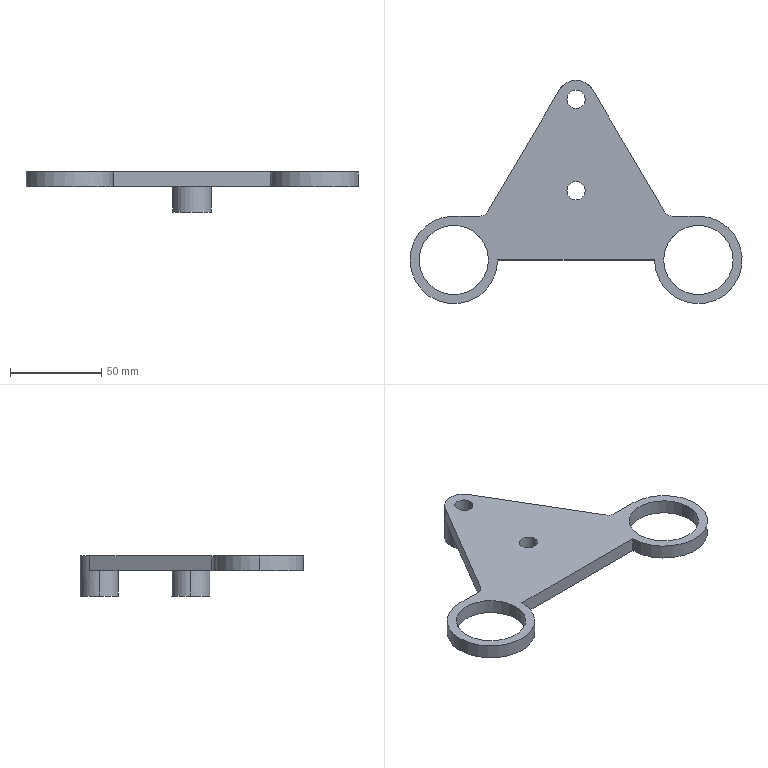Part | SolidWorks | features Extrusion 1, ICE 1 | 1 solid | 26 faces | box 182 x 122.5 x 22 mm | volume 68800 mm3 | cylinder 17 | plane 9 | commonest cylinder face diameters 10 x6 21 x4 38 x4 48 x3
STEP:
#1=CARTESIAN_POINT('',(-10.5,38.,-14.));
#2=VERTEX_POINT('',#1);
#3=CARTESIAN_POINT('',(10.5,38.,-14.));
#4=VERTEX_POINT('',#3);
#5=CARTESIAN_POINT('',(0.,38.,-14.));
#6=DIRECTION('',(0.,0.,-1.));
#7=DIRECTION('',(-1.,0.,0.));
#8=AXIS2_PLACEMENT_3D('',#5,#6,#7);
#9=CIRCLE('',#8,10.5);
#10=EDGE_CURVE('',#2,#4,#9,.T.);
#11=ORIENTED_EDGE('',*,*,#10,.F.);
#12=CARTESIAN_POINT('',(-10.5,38.,0.));
#13=VERTEX_POINT('',#12);
#14=CARTESIAN_POINT('',(-10.5,38.,-14.));
#15=DIRECTION('',(0.,0.,1.));
#16=VECTOR('',#15,1000.);
#17=LINE('',#14,#16);
#18=EDGE_CURVE('',#2,#13,#17,.T.);
#19=ORIENTED_EDGE('',*,*,#18,.T.);
#20=CARTESIAN_POINT('',(10.5,38.,0.));
#21=VERTEX_POINT('',#20);
#22=CARTESIAN_POINT('',(0.,38.,0.));
#23=DIRECTION('',(0.,0.,-1.));
#24=DIRECTION('',(1.,0.,0.));
#25=AXIS2_PLACEMENT_3D('',#22,#23,#24);
#26=CIRCLE('',#25,10.5);
#27=EDGE_CURVE('',#13,#21,#26,.T.);
#28=ORIENTED_EDGE('',*,*,#27,.T.);
#29=CARTESIAN_POINT('',(10.5,38.,-14.));
#30=DIRECTION('',(0.,0.,1.));
#31=VECTOR('',#30,1000.);
#32=LINE('',#29,#31);
#33=EDGE_CURVE('',#4,#21,#32,.T.);
#34=ORIENTED_EDGE('',*,*,#33,.F.);
#35=EDGE_LOOP('',(#11,#19,#28,#34));
#36=FACE_OUTER_BOUND('',#35,.T.);
#37=CARTESIAN_POINT('',(0.,38.,-14.));
#38=DIRECTION('',(0.,0.,1.));
#39=DIRECTION('',(1.,0.,0.));
#40=AXIS2_PLACEMENT_3D('',#37,#38,#39);
#41=CYLINDRICAL_SURFACE('',#40,10.5);
#42=ADVANCED_FACE('',(#36),#41,.T.);
#43=CARTESIAN_POINT('',(-5.,38.,8.));
#44=VERTEX_POINT('',#43);
#45=CARTESIAN_POINT('',(5.,38.,8.));
#46=VERTEX_POINT('',#45);
#47=CARTESIAN_POINT('',(0.,38.,8.));
#48=DIRECTION('',(0.,0.,1.));
#49=DIRECTION('',(1.,0.,0.));
#50=AXIS2_PLACEMENT_3D('',#47,#48,#49);
#51=CIRCLE('',#50,5.);
#52=EDGE_CURVE('',#44,#46,#51,.T.);
#53=ORIENTED_EDGE('',*,*,#52,.T.);
#54=CARTESIAN_POINT('',(5.,38.,-14.));
#55=VERTEX_POINT('',#54);
#56=CARTESIAN_POINT('',(5.,38.,8.));
#57=DIRECTION('',(0.,0.,-1.));
#58=VECTOR('',#57,1000.);
#59=LINE('',#56,#58);
#60=EDGE_CURVE('',#46,#55,#59,.T.);
#61=ORIENTED_EDGE('',*,*,#60,.T.);
#62=CARTESIAN_POINT('',(-5.,38.,-14.));
#63=VERTEX_POINT('',#62);
#64=CARTESIAN_POINT('',(0.,38.,-14.));
#65=DIRECTION('',(0.,0.,-1.));
#66=DIRECTION('',(-1.,0.,0.));
#67=AXIS2_PLACEMENT_3D('',#64,#65,#66);
#68=CIRCLE('',#67,5.);
#69=EDGE_CURVE('',#55,#63,#68,.T.);
#70=ORIENTED_EDGE('',*,*,#69,.T.);
#71=CARTESIAN_POINT('',(-5.,38.,8.));
#72=DIRECTION('',(0.,0.,-1.));
#73=VECTOR('',#72,1000.);
#74=LINE('',#71,#73);
#75=EDGE_CURVE('',#44,#63,#74,.T.);
#76=ORIENTED_EDGE('',*,*,#75,.F.);
#77=EDGE_LOOP('',(#53,#61,#70,#76));
#78=FACE_OUTER_BOUND('',#77,.T.);
#79=CARTESIAN_POINT('',(0.,38.,8.));
#80=DIRECTION('',(0.,0.,-1.));
#81=DIRECTION('',(-1.,0.,0.));
#82=AXIS2_PLACEMENT_3D('',#79,#80,#81);
#83=CYLINDRICAL_SURFACE('',#82,5.);
#84=ADVANCED_FACE('',(#78),#83,.F.);
#85=CARTESIAN_POINT('',(-5.,88.,8.));
#86=VERTEX_POINT('',#85);
#87=CARTESIAN_POINT('',(5.,88.,8.));
#88=VERTEX_POINT('',#87);
#89=CARTESIAN_POINT('',(0.,88.,8.));
#90=DIRECTION('',(0.,0.,1.));
#91=DIRECTION('',(1.,0.,0.));
#92=AXIS2_PLACEMENT_3D('',#89,#90,#91);
#93=CIRCLE('',#92,5.);
#94=EDGE_CURVE('',#86,#88,#93,.T.);
#95=ORIENTED_EDGE('',*,*,#94,.T.);
#96=CARTESIAN_POINT('',(5.,88.,-14.));
#97=VERTEX_POINT('',#96);
#98=CARTESIAN_POINT('',(5.,88.,8.));
#99=DIRECTION('',(0.,0.,-1.));
#100=VECTOR('',#99,1000.);
#101=LINE('',#98,#100);
#102=EDGE_CURVE('',#88,#97,#101,.T.);
#103=ORIENTED_EDGE('',*,*,#102,.T.);
#104=CARTESIAN_POINT('',(-5.,88.,-14.));
#105=VERTEX_POINT('',#104);
#106=CARTESIAN_POINT('',(0.,88.,-14.));
#107=DIRECTION('',(0.,0.,-1.));
#108=DIRECTION('',(-1.,0.,0.));
#109=AXIS2_PLACEMENT_3D('',#106,#107,#108);
#110=CIRCLE('',#109,5.);
#111=EDGE_CURVE('',#97,#105,#110,.T.);
#112=ORIENTED_EDGE('',*,*,#111,.T.);
#113=CARTESIAN_POINT('',(-5.,88.,8.));
#114=DIRECTION('',(0.,0.,-1.));
#115=VECTOR('',#114,1000.);
#116=LINE('',#113,#115);
#117=EDGE_CURVE('',#86,#105,#116,.T.);
#118=ORIENTED_EDGE('',*,*,#117,.F.);
#119=EDGE_LOOP('',(#95,#103,#112,#118));
#120=FACE_OUTER_BOUND('',#119,.T.);
#121=CARTESIAN_POINT('',(0.,88.,8.));
#122=DIRECTION('',(0.,0.,-1.));
#123=DIRECTION('',(-1.,0.,0.));
#124=AXIS2_PLACEMENT_3D('',#121,#122,#123);
#125=CYLINDRICAL_SURFACE('',#124,5.);
#126=ADVANCED_FACE('',(#120),#125,.F.);
#127=CARTESIAN_POINT('',(86.,0.,8.));
#128=VERTEX_POINT('',#127);
#129=CARTESIAN_POINT('',(48.,0.,8.));
#130=VERTEX_POINT('',#129);
#131=CARTESIAN_POINT('',(67.,0.,8.));
#132=DIRECTION('',(0.,0.,-1.));
#133=DIRECTION('',(1.,0.,0.));
#134=AXIS2_PLACEMENT_3D('',#131,#132,#133);
#135=CIRCLE('',#134,19.);
#136=EDGE_CURVE('',#128,#130,#135,.T.);
#137=ORIENTED_EDGE('',*,*,#136,.F.);
#138=CARTESIAN_POINT('',(86.,0.,0.));
#139=VERTEX_POINT('',#138);
#140=CARTESIAN_POINT('',(86.,0.,8.));
#141=DIRECTION('',(0.,0.,-1.));
#142=VECTOR('',#141,1000.);
#143=LINE('',#140,#142);
#144=EDGE_CURVE('',#128,#139,#143,.T.);
#145=ORIENTED_EDGE('',*,*,#144,.T.);
#146=CARTESIAN_POINT('',(48.,0.,0.));
#147=VERTEX_POINT('',#146);
#148=CARTESIAN_POINT('',(67.,0.,0.));
#149=DIRECTION('',(0.,0.,-1.));
#150=DIRECTION('',(1.,0.,0.));
#151=AXIS2_PLACEMENT_3D('',#148,#149,#150);
#152=CIRCLE('',#151,19.);
#153=EDGE_CURVE('',#139,#147,#152,.T.);
#154=ORIENTED_EDGE('',*,*,#153,.T.);
#155=CARTESIAN_POINT('',(48.,0.,8.));
#156=DIRECTION('',(0.,0.,-1.));
#157=VECTOR('',#156,1000.);
#158=LINE('',#155,#157);
#159=EDGE_CURVE('',#130,#147,#158,.T.);
#160=ORIENTED_EDGE('',*,*,#159,.F.);
#161=EDGE_LOOP('',(#137,#145,#154,#160));
#162=FACE_OUTER_BOUND('',#161,.T.);
#163=CARTESIAN_POINT('',(67.,0.,8.));
#164=DIRECTION('',(0.,0.,-1.));
#165=DIRECTION('',(-1.,0.,0.));
#166=AXIS2_PLACEMENT_3D('',#163,#164,#165);
#167=CYLINDRICAL_SURFACE('',#166,19.);
#168=ADVANCED_FACE('',(#162),#167,.F.);
#169=CARTESIAN_POINT('',(-86.,0.,8.));
#170=VERTEX_POINT('',#169);
#171=CARTESIAN_POINT('',(-48.,0.,8.));
#172=VERTEX_POINT('',#171);
#173=CARTESIAN_POINT('',(-67.,0.,8.));
#174=DIRECTION('',(0.,0.,1.));
#175=DIRECTION('',(1.,0.,0.));
#176=AXIS2_PLACEMENT_3D('',#173,#174,#175);
#177=CIRCLE('',#176,19.);
#178=EDGE_CURVE('',#170,#172,#177,.T.);
#179=ORIENTED_EDGE('',*,*,#178,.T.);
#180=CARTESIAN_POINT('',(-48.,0.,0.));
#181=VERTEX_POINT('',#180);
#182=CARTESIAN_POINT('',(-48.,0.,8.));
#183=DIRECTION('',(0.,0.,-1.));
#184=VECTOR('',#183,1000.);
#185=LINE('',#182,#184);
#186=EDGE_CURVE('',#172,#181,#185,.T.);
#187=ORIENTED_EDGE('',*,*,#186,.T.);
#188=CARTESIAN_POINT('',(-86.,0.,0.));
#189=VERTEX_POINT('',#188);
#190=CARTESIAN_POINT('',(-67.,0.,0.));
#191=DIRECTION('',(0.,0.,1.));
#192=DIRECTION('',(1.,0.,0.));
#193=AXIS2_PLACEMENT_3D('',#190,#191,#192);
#194=CIRCLE('',#193,19.);
#195=EDGE_CURVE('',#189,#181,#194,.T.);
#196=ORIENTED_EDGE('',*,*,#195,.F.);
#197=CARTESIAN_POINT('',(-86.,0.,8.));
#198=DIRECTION('',(0.,0.,-1.));
#199=VECTOR('',#198,1000.);
#200=LINE('',#197,#199);
#201=EDGE_CURVE('',#170,#189,#200,.T.);
#202=ORIENTED_EDGE('',*,*,#201,.F.);
#203=EDGE_LOOP('',(#179,#187,#196,#202));
#204=FACE_OUTER_BOUND('',#203,.T.);
#205=CARTESIAN_POINT('',(-67.,0.,8.));
#206=DIRECTION('',(0.,0.,-1.));
#207=DIRECTION('',(-1.,0.,0.));
#208=AXIS2_PLACEMENT_3D('',#205,#206,#207);
#209=CYLINDRICAL_SURFACE('',#208,19.);
#210=ADVANCED_FACE('',(#204),#209,.F.);
#211=CARTESIAN_POINT('',(-91.,0.,8.));
#212=VERTEX_POINT('',#211);
#213=CARTESIAN_POINT('',(-43.,0.,8.));
#214=VERTEX_POINT('',#213);
#215=CARTESIAN_POINT('',(-67.,0.,8.));
#216=DIRECTION('',(0.,0.,1.));
#217=DIRECTION('',(1.,0.,0.));
#218=AXIS2_PLACEMENT_3D('',#215,#216,#217);
#219=CIRCLE('',#218,24.);
#220=EDGE_CURVE('',#212,#214,#219,.T.);
#221=ORIENTED_EDGE('',*,*,#220,.F.);
#222=CARTESIAN_POINT('',(-91.,0.,0.));
#223=VERTEX_POINT('',#222);
#224=CARTESIAN_POINT('',(-91.,0.,8.));
#225=DIRECTION('',(0.,0.,-1.));
#226=VECTOR('',#225,1000.);
#227=LINE('',#224,#226);
#228=EDGE_CURVE('',#212,#223,#227,.T.);
#229=ORIENTED_EDGE('',*,*,#228,.T.);
#230=CARTESIAN_POINT('',(-43.,0.,0.));
#231=VERTEX_POINT('',#230);
#232=CARTESIAN_POINT('',(-67.,0.,0.));
#233=DIRECTION('',(0.,0.,1.));
#234=DIRECTION('',(1.,0.,0.));
#235=AXIS2_PLACEMENT_3D('',#232,#233,#234);
#236=CIRCLE('',#235,24.);
#237=EDGE_CURVE('',#223,#231,#236,.T.);
#238=ORIENTED_EDGE('',*,*,#237,.T.);
#239=CARTESIAN_POINT('',(-43.,0.,8.));
#240=DIRECTION('',(0.,0.,-1.));
#241=VECTOR('',#240,1000.);
#242=LINE('',#239,#241);
#243=EDGE_CURVE('',#214,#231,#242,.T.);
#244=ORIENTED_EDGE('',*,*,#243,.F.);
#245=EDGE_LOOP('',(#221,#229,#238,#244));
#246=FACE_OUTER_BOUND('',#245,.T.);
#247=CARTESIAN_POINT('',(-67.,0.,8.));
#248=DIRECTION('',(0.,0.,-1.));
#249=DIRECTION('',(-1.,0.,0.));
#250=AXIS2_PLACEMENT_3D('',#247,#248,#249);
#251=CYLINDRICAL_SURFACE('',#250,24.);
#252=ADVANCED_FACE('',(#246),#251,.T.);
#253=CARTESIAN_POINT('',(9.093,93.25,0.));
#254=VERTEX_POINT('',#253);
#255=CARTESIAN_POINT('',(10.5,88.,0.));
#256=VERTEX_POINT('',#255);
#257=CARTESIAN_POINT('',(0.,88.,0.));
#258=DIRECTION('',(0.,0.,-1.));
#259=DIRECTION('',(-1.,0.,0.));
#260=AXIS2_PLACEMENT_3D('',#257,#258,#259);
#261=CIRCLE('',#260,10.5);
#262=EDGE_CURVE('',#254,#256,#261,.T.);
#263=ORIENTED_EDGE('',*,*,#262,.T.);
#264=CARTESIAN_POINT('',(10.5,88.,-14.));
#265=VERTEX_POINT('',#264);
#266=CARTESIAN_POINT('',(10.5,88.,8.));
#267=DIRECTION('',(0.,0.,-1.));
#268=VECTOR('',#267,1000.);
#269=LINE('',#266,#268);
#270=EDGE_CURVE('',#256,#265,#269,.T.);
#271=ORIENTED_EDGE('',*,*,#270,.T.);
#272=CARTESIAN_POINT('',(-10.5,88.,-14.));
#273=VERTEX_POINT('',#272);
#274=CARTESIAN_POINT('',(0.,88.,-14.));
#275=DIRECTION('',(0.,0.,-1.));
#276=DIRECTION('',(-1.,0.,0.));
#277=AXIS2_PLACEMENT_3D('',#274,#275,#276);
#278=CIRCLE('',#277,10.5);
#279=EDGE_CURVE('',#273,#265,#278,.T.);
#280=ORIENTED_EDGE('',*,*,#279,.F.);
#281=CARTESIAN_POINT('',(-10.5,88.,0.));
#282=VERTEX_POINT('',#281);
#283=CARTESIAN_POINT('',(-10.5,88.,8.));
#284=DIRECTION('',(0.,0.,-1.));
#285=VECTOR('',#284,1000.);
#286=LINE('',#283,#285);
#287=EDGE_CURVE('',#282,#273,#286,.T.);
#288=ORIENTED_EDGE('',*,*,#287,.F.);
#289=CARTESIAN_POINT('',(-9.093,93.25,0.));
#290=VERTEX_POINT('',#289);
#291=CARTESIAN_POINT('',(0.,88.,0.));
#292=DIRECTION('',(0.,0.,-1.));
#293=DIRECTION('',(-1.,0.,0.));
#294=AXIS2_PLACEMENT_3D('',#291,#292,#293);
#295=CIRCLE('',#294,10.5);
#296=EDGE_CURVE('',#282,#290,#295,.T.);
#297=ORIENTED_EDGE('',*,*,#296,.T.);
#298=CARTESIAN_POINT('',(-9.093,93.25,8.));
#299=VERTEX_POINT('',#298);
#300=CARTESIAN_POINT('',(-9.093,93.25,8.));
#301=DIRECTION('',(0.,0.,-1.));
#302=VECTOR('',#301,1000.);
#303=LINE('',#300,#302);
#304=EDGE_CURVE('',#299,#290,#303,.T.);
#305=ORIENTED_EDGE('',*,*,#304,.F.);
#306=CARTESIAN_POINT('',(9.093,93.25,8.));
#307=VERTEX_POINT('',#306);
#308=CARTESIAN_POINT('',(0.,88.,8.));
#309=DIRECTION('',(0.,0.,1.));
#310=DIRECTION('',(1.,0.,0.));
#311=AXIS2_PLACEMENT_3D('',#308,#309,#310);
#312=CIRCLE('',#311,10.5);
#313=EDGE_CURVE('',#307,#299,#312,.T.);
#314=ORIENTED_EDGE('',*,*,#313,.F.);
#315=CARTESIAN_POINT('',(9.093,93.25,8.));
#316=DIRECTION('',(0.,0.,-1.));
#317=VECTOR('',#316,1000.);
#318=LINE('',#315,#317);
#319=EDGE_CURVE('',#307,#254,#318,.T.);
#320=ORIENTED_EDGE('',*,*,#319,.T.);
#321=EDGE_LOOP('',(#263,#271,#280,#288,#297,#305,#314,#320));
#322=FACE_OUTER_BOUND('',#321,.T.);
#323=CARTESIAN_POINT('',(0.,88.,8.));
#324=DIRECTION('',(0.,0.,-1.));
#325=DIRECTION('',(-1.,0.,0.));
#326=AXIS2_PLACEMENT_3D('',#323,#324,#325);
#327=CYLINDRICAL_SURFACE('',#326,10.5);
#328=ADVANCED_FACE('',(#322),#327,.T.);
#329=ORIENTED_EDGE('',*,*,#195,.T.);
#330=CARTESIAN_POINT('',(-67.,0.,0.));
#331=DIRECTION('',(0.,0.,1.));
#332=DIRECTION('',(1.,0.,0.));
#333=AXIS2_PLACEMENT_3D('',#330,#331,#332);
#334=CIRCLE('',#333,19.);
#335=EDGE_CURVE('',#181,#189,#334,.T.);
#336=ORIENTED_EDGE('',*,*,#335,.T.);
#337=EDGE_LOOP('',(#329,#336));
#338=FACE_BOUND('',#337,.T.);
#339=CARTESIAN_POINT('',(67.,0.,0.));
#340=DIRECTION('',(0.,0.,-1.));
#341=DIRECTION('',(1.,0.,0.));
#342=AXIS2_PLACEMENT_3D('',#339,#340,#341);
#343=CIRCLE('',#342,19.);
#344=EDGE_CURVE('',#147,#139,#343,.T.);
#345=ORIENTED_EDGE('',*,*,#344,.F.);
#346=ORIENTED_EDGE('',*,*,#153,.F.);
#347=EDGE_LOOP('',(#345,#346));
#348=FACE_BOUND('',#347,.T.);
#349=ORIENTED_EDGE('',*,*,#262,.F.);
#350=CARTESIAN_POINT('',(48.477,26.46,0.));
#351=VERTEX_POINT('',#350);
#352=CARTESIAN_POINT('',(47.547,28.037,0.));
#353=DIRECTION('',(0.5079,-0.8614,0.));
#354=VECTOR('',#353,1000.);
#355=LINE('',#352,#354);
#356=EDGE_CURVE('',#254,#351,#355,.T.);
#357=ORIENTED_EDGE('',*,*,#356,.T.);
#358=CARTESIAN_POINT('',(52.82,24.,0.));
#359=VERTEX_POINT('',#358);
#360=CARTESIAN_POINT('',(52.785,29.,0.));
#361=DIRECTION('',(0.,0.,-1.));
#362=DIRECTION('',(1.,0.,0.));
#363=AXIS2_PLACEMENT_3D('',#360,#361,#362);
#364=CIRCLE('',#363,5.);
#365=EDGE_CURVE('',#359,#351,#364,.T.);
#366=ORIENTED_EDGE('',*,*,#365,.F.);
#367=CARTESIAN_POINT('',(67.,24.,0.));
#368=VERTEX_POINT('',#367);
#369=CARTESIAN_POINT('',(0.,24.,0.));
#370=DIRECTION('',(-1.,0.,0.));
#371=VECTOR('',#370,1000.);
#372=LINE('',#369,#371);
#373=EDGE_CURVE('',#368,#359,#372,.T.);
#374=ORIENTED_EDGE('',*,*,#373,.F.);
#375=CARTESIAN_POINT('',(43.,0.,0.));
#376=VERTEX_POINT('',#375);
#377=CARTESIAN_POINT('',(67.,0.,0.));
#378=DIRECTION('',(0.,0.,-1.));
#379=DIRECTION('',(1.,0.,0.));
#380=AXIS2_PLACEMENT_3D('',#377,#378,#379);
#381=CIRCLE('',#380,24.);
#382=EDGE_CURVE('',#368,#376,#381,.T.);
#383=ORIENTED_EDGE('',*,*,#382,.T.);
#384=CARTESIAN_POINT('',(0.,0.,0.));
#385=DIRECTION('',(1.,0.,0.));
#386=VECTOR('',#385,1000.);
#387=LINE('',#384,#386);
#388=EDGE_CURVE('',#231,#376,#387,.T.);
#389=ORIENTED_EDGE('',*,*,#388,.F.);
#390=ORIENTED_EDGE('',*,*,#237,.F.);
#391=CARTESIAN_POINT('',(-67.,24.,0.));
#392=VERTEX_POINT('',#391);
#393=CARTESIAN_POINT('',(-67.,0.,0.));
#394=DIRECTION('',(0.,0.,1.));
#395=DIRECTION('',(1.,0.,0.));
#396=AXIS2_PLACEMENT_3D('',#393,#394,#395);
#397=CIRCLE('',#396,24.);
#398=EDGE_CURVE('',#392,#223,#397,.T.);
#399=ORIENTED_EDGE('',*,*,#398,.F.);
#400=CARTESIAN_POINT('',(-52.82,24.,0.));
#401=VERTEX_POINT('',#400);
#402=CARTESIAN_POINT('',(0.,24.,0.));
#403=DIRECTION('',(1.,0.,0.));
#404=VECTOR('',#403,1000.);
#405=LINE('',#402,#404);
#406=EDGE_CURVE('',#392,#401,#405,.T.);
#407=ORIENTED_EDGE('',*,*,#406,.T.);
#408=CARTESIAN_POINT('',(-48.477,26.46,0.));
#409=VERTEX_POINT('',#408);
#410=CARTESIAN_POINT('',(-52.785,29.,0.));
#411=DIRECTION('',(0.,0.,1.));
#412=DIRECTION('',(1.,0.,0.));
#413=AXIS2_PLACEMENT_3D('',#410,#411,#412);
#414=CIRCLE('',#413,5.);
#415=EDGE_CURVE('',#401,#409,#414,.T.);
#416=ORIENTED_EDGE('',*,*,#415,.T.);
#417=CARTESIAN_POINT('',(-47.547,28.037,0.));
#418=DIRECTION('',(-0.5079,-0.8614,0.));
#419=VECTOR('',#418,1000.);
#420=LINE('',#417,#419);
#421=EDGE_CURVE('',#290,#409,#420,.T.);
#422=ORIENTED_EDGE('',*,*,#421,.F.);
#423=ORIENTED_EDGE('',*,*,#296,.F.);
#424=CARTESIAN_POINT('',(0.,88.,0.));
#425=DIRECTION('',(0.,0.,-1.));
#426=DIRECTION('',(-1.,0.,0.));
#427=AXIS2_PLACEMENT_3D('',#424,#425,#426);
#428=CIRCLE('',#427,10.5);
#429=EDGE_CURVE('',#256,#282,#428,.T.);
#430=ORIENTED_EDGE('',*,*,#429,.F.);
#431=EDGE_LOOP('',(#349,#357,#366,#374,#383,#389,#390,#399,#407,#416,#422,#423,#430));
#432=FACE_OUTER_BOUND('',#431,.T.);
#433=CARTESIAN_POINT('',(0.,38.,0.));
#434=DIRECTION('',(0.,0.,-1.));
#435=DIRECTION('',(1.,0.,0.));
#436=AXIS2_PLACEMENT_3D('',#433,#434,#435);
#437=CIRCLE('',#436,10.5);
#438=EDGE_CURVE('',#21,#13,#437,.T.);
#439=ORIENTED_EDGE('',*,*,#438,.F.);
#440=ORIENTED_EDGE('',*,*,#27,.F.);
#441=EDGE_LOOP('',(#439,#440));
#442=FACE_BOUND('',#441,.T.);
#443=CARTESIAN_POINT('',(0.,0.,0.));
#444=DIRECTION('',(0.,0.,1.));
#445=DIRECTION('',(1.,0.,0.));
#446=AXIS2_PLACEMENT_3D('',#443,#444,#445);
#447=PLANE('',#446);
#448=ADVANCED_FACE('',(#338,#348,#432,#442),#447,.F.);
#449=ORIENTED_EDGE('',*,*,#373,.T.);
#450=CARTESIAN_POINT('',(52.82,24.,8.));
#451=VERTEX_POINT('',#450);
#452=CARTESIAN_POINT('',(52.82,24.,8.));
#453=DIRECTION('',(0.,0.,-1.));
#454=VECTOR('',#453,1000.);
#455=LINE('',#452,#454);
#456=EDGE_CURVE('',#451,#359,#455,.T.);
#457=ORIENTED_EDGE('',*,*,#456,.F.);
#458=CARTESIAN_POINT('',(67.,24.,8.));
#459=VERTEX_POINT('',#458);
#460=CARTESIAN_POINT('',(0.,24.,8.));
#461=DIRECTION('',(-1.,0.,0.));
#462=VECTOR('',#461,1000.);
#463=LINE('',#460,#462);
#464=EDGE_CURVE('',#459,#451,#463,.T.);
#465=ORIENTED_EDGE('',*,*,#464,.F.);
#466=CARTESIAN_POINT('',(67.,24.,8.));
#467=DIRECTION('',(0.,0.,-1.));
#468=VECTOR('',#467,1000.);
#469=LINE('',#466,#468);
#470=EDGE_CURVE('',#459,#368,#469,.T.);
#471=ORIENTED_EDGE('',*,*,#470,.T.);
#472=EDGE_LOOP('',(#449,#457,#465,#471));
#473=FACE_OUTER_BOUND('',#472,.T.);
#474=CARTESIAN_POINT('',(0.,24.,8.));
#475=DIRECTION('',(0.,-1.,0.));
#476=DIRECTION('',(1.,0.,0.));
#477=AXIS2_PLACEMENT_3D('',#474,#475,#476);
#478=PLANE('',#477);
#479=ADVANCED_FACE('',(#473),#478,.F.);
#480=ORIENTED_EDGE('',*,*,#365,.T.);
#481=CARTESIAN_POINT('',(48.477,26.46,8.));
#482=VERTEX_POINT('',#481);
#483=CARTESIAN_POINT('',(48.477,26.46,8.));
#484=DIRECTION('',(0.,0.,-1.));
#485=VECTOR('',#484,1000.);
#486=LINE('',#483,#485);
#487=EDGE_CURVE('',#482,#351,#486,.T.);
#488=ORIENTED_EDGE('',*,*,#487,.F.);
#489=CARTESIAN_POINT('',(52.785,29.,8.));
#490=DIRECTION('',(0.,0.,-1.));
#491=DIRECTION('',(1.,0.,0.));
#492=AXIS2_PLACEMENT_3D('',#489,#490,#491);
#493=CIRCLE('',#492,5.);
#494=EDGE_CURVE('',#451,#482,#493,.T.);
#495=ORIENTED_EDGE('',*,*,#494,.F.);
#496=ORIENTED_EDGE('',*,*,#456,.T.);
#497=EDGE_LOOP('',(#480,#488,#495,#496));
#498=FACE_OUTER_BOUND('',#497,.T.);
#499=CARTESIAN_POINT('',(52.785,29.,8.));
#500=DIRECTION('',(0.,0.,-1.));
#501=DIRECTION('',(-1.,0.,0.));
#502=AXIS2_PLACEMENT_3D('',#499,#500,#501);
#503=CYLINDRICAL_SURFACE('',#502,5.);
#504=ADVANCED_FACE('',(#498),#503,.F.);
#505=ORIENTED_EDGE('',*,*,#356,.F.);
#506=ORIENTED_EDGE('',*,*,#319,.F.);
#507=CARTESIAN_POINT('',(47.547,28.037,8.));
#508=DIRECTION('',(0.5079,-0.8614,0.));
#509=VECTOR('',#508,1000.);
#510=LINE('',#507,#509);
#511=EDGE_CURVE('',#307,#482,#510,.T.);
#512=ORIENTED_EDGE('',*,*,#511,.T.);
#513=ORIENTED_EDGE('',*,*,#487,.T.);
#514=EDGE_LOOP('',(#505,#506,#512,#513));
#515=FACE_OUTER_BOUND('',#514,.T.);
#516=CARTESIAN_POINT('',(47.547,28.037,8.));
#517=DIRECTION('',(0.8614,0.5079,0.));
#518=DIRECTION('',(-0.5079,0.8614,0.));
#519=AXIS2_PLACEMENT_3D('',#516,#517,#518);
#520=PLANE('',#519);
#521=ADVANCED_FACE('',(#515),#520,.T.);
#522=ORIENTED_EDGE('',*,*,#270,.F.);
#523=ORIENTED_EDGE('',*,*,#429,.T.);
#524=ORIENTED_EDGE('',*,*,#287,.T.);
#525=CARTESIAN_POINT('',(0.,88.,-14.));
#526=DIRECTION('',(0.,0.,-1.));
#527=DIRECTION('',(-1.,0.,0.));
#528=AXIS2_PLACEMENT_3D('',#525,#526,#527);
#529=CIRCLE('',#528,10.5);
#530=EDGE_CURVE('',#265,#273,#529,.T.);
#531=ORIENTED_EDGE('',*,*,#530,.F.);
#532=EDGE_LOOP('',(#522,#523,#524,#531));
#533=FACE_OUTER_BOUND('',#532,.T.);
#534=CARTESIAN_POINT('',(0.,88.,8.));
#535=DIRECTION('',(0.,0.,-1.));
#536=DIRECTION('',(-1.,0.,0.));
#537=AXIS2_PLACEMENT_3D('',#534,#535,#536);
#538=CYLINDRICAL_SURFACE('',#537,10.5);
#539=ADVANCED_FACE('',(#533),#538,.T.);
#540=ORIENTED_EDGE('',*,*,#421,.T.);
#541=CARTESIAN_POINT('',(-48.477,26.46,8.));
#542=VERTEX_POINT('',#541);
#543=CARTESIAN_POINT('',(-48.477,26.46,8.));
#544=DIRECTION('',(0.,0.,-1.));
#545=VECTOR('',#544,1000.);
#546=LINE('',#543,#545);
#547=EDGE_CURVE('',#542,#409,#546,.T.);
#548=ORIENTED_EDGE('',*,*,#547,.F.);
#549=CARTESIAN_POINT('',(-47.547,28.037,8.));
#550=DIRECTION('',(-0.5079,-0.8614,0.));
#551=VECTOR('',#550,1000.);
#552=LINE('',#549,#551);
#553=EDGE_CURVE('',#299,#542,#552,.T.);
#554=ORIENTED_EDGE('',*,*,#553,.F.);
#555=ORIENTED_EDGE('',*,*,#304,.T.);
#556=EDGE_LOOP('',(#540,#548,#554,#555));
#557=FACE_OUTER_BOUND('',#556,.T.);
#558=CARTESIAN_POINT('',(-47.547,28.037,8.));
#559=DIRECTION('',(0.8614,-0.5079,0.));
#560=DIRECTION('',(0.5079,0.8614,0.));
#561=AXIS2_PLACEMENT_3D('',#558,#559,#560);
#562=PLANE('',#561);
#563=ADVANCED_FACE('',(#557),#562,.F.);
#564=ORIENTED_EDGE('',*,*,#415,.F.);
#565=CARTESIAN_POINT('',(-52.82,24.,8.));
#566=VERTEX_POINT('',#565);
#567=CARTESIAN_POINT('',(-52.82,24.,8.));
#568=DIRECTION('',(0.,0.,-1.));
#569=VECTOR('',#568,1000.);
#570=LINE('',#567,#569);
#571=EDGE_CURVE('',#566,#401,#570,.T.);
#572=ORIENTED_EDGE('',*,*,#571,.F.);
#573=CARTESIAN_POINT('',(-52.785,29.,8.));
#574=DIRECTION('',(0.,0.,1.));
#575=DIRECTION('',(1.,0.,0.));
#576=AXIS2_PLACEMENT_3D('',#573,#574,#575);
#577=CIRCLE('',#576,5.);
#578=EDGE_CURVE('',#566,#542,#577,.T.);
#579=ORIENTED_EDGE('',*,*,#578,.T.);
#580=ORIENTED_EDGE('',*,*,#547,.T.);
#581=EDGE_LOOP('',(#564,#572,#579,#580));
#582=FACE_OUTER_BOUND('',#581,.T.);
#583=CARTESIAN_POINT('',(-52.785,29.,8.));
#584=DIRECTION('',(0.,0.,-1.));
#585=DIRECTION('',(-1.,0.,0.));
#586=AXIS2_PLACEMENT_3D('',#583,#584,#585);
#587=CYLINDRICAL_SURFACE('',#586,5.);
#588=ADVANCED_FACE('',(#582),#587,.F.);
#589=ORIENTED_EDGE('',*,*,#406,.F.);
#590=CARTESIAN_POINT('',(-67.,24.,8.));
#591=VERTEX_POINT('',#590);
#592=CARTESIAN_POINT('',(-67.,24.,8.));
#593=DIRECTION('',(0.,0.,-1.));
#594=VECTOR('',#593,1000.);
#595=LINE('',#592,#594);
#596=EDGE_CURVE('',#591,#392,#595,.T.);
#597=ORIENTED_EDGE('',*,*,#596,.F.);
#598=CARTESIAN_POINT('',(0.,24.,8.));
#599=DIRECTION('',(1.,0.,0.));
#600=VECTOR('',#599,1000.);
#601=LINE('',#598,#600);
#602=EDGE_CURVE('',#591,#566,#601,.T.);
#603=ORIENTED_EDGE('',*,*,#602,.T.);
#604=ORIENTED_EDGE('',*,*,#571,.T.);
#605=EDGE_LOOP('',(#589,#597,#603,#604));
#606=FACE_OUTER_BOUND('',#605,.T.);
#607=CARTESIAN_POINT('',(0.,24.,8.));
#608=DIRECTION('',(0.,1.,0.));
#609=DIRECTION('',(-1.,0.,0.));
#610=AXIS2_PLACEMENT_3D('',#607,#608,#609);
#611=PLANE('',#610);
#612=ADVANCED_FACE('',(#606),#611,.T.);
#613=ORIENTED_EDGE('',*,*,#228,.F.);
#614=CARTESIAN_POINT('',(-67.,0.,8.));
#615=DIRECTION('',(0.,0.,1.));
#616=DIRECTION('',(1.,0.,0.));
#617=AXIS2_PLACEMENT_3D('',#614,#615,#616);
#618=CIRCLE('',#617,24.);
#619=EDGE_CURVE('',#591,#212,#618,.T.);
#620=ORIENTED_EDGE('',*,*,#619,.F.);
#621=ORIENTED_EDGE('',*,*,#596,.T.);
#622=ORIENTED_EDGE('',*,*,#398,.T.);
#623=EDGE_LOOP('',(#613,#620,#621,#622));
#624=FACE_OUTER_BOUND('',#623,.T.);
#625=CARTESIAN_POINT('',(-67.,0.,8.));
#626=DIRECTION('',(0.,0.,-1.));
#627=DIRECTION('',(-1.,0.,0.));
#628=AXIS2_PLACEMENT_3D('',#625,#626,#627);
#629=CYLINDRICAL_SURFACE('',#628,24.);
#630=ADVANCED_FACE('',(#624),#629,.T.);
#631=ORIENTED_EDGE('',*,*,#388,.T.);
#632=CARTESIAN_POINT('',(43.,0.,8.));
#633=VERTEX_POINT('',#632);
#634=CARTESIAN_POINT('',(43.,0.,8.));
#635=DIRECTION('',(0.,0.,-1.));
#636=VECTOR('',#635,1000.);
#637=LINE('',#634,#636);
#638=EDGE_CURVE('',#633,#376,#637,.T.);
#639=ORIENTED_EDGE('',*,*,#638,.F.);
#640=CARTESIAN_POINT('',(0.,0.,8.));
#641=DIRECTION('',(1.,0.,0.));
#642=VECTOR('',#641,1000.);
#643=LINE('',#640,#642);
#644=EDGE_CURVE('',#214,#633,#643,.T.);
#645=ORIENTED_EDGE('',*,*,#644,.F.);
#646=ORIENTED_EDGE('',*,*,#243,.T.);
#647=EDGE_LOOP('',(#631,#639,#645,#646));
#648=FACE_OUTER_BOUND('',#647,.T.);
#649=CARTESIAN_POINT('',(0.,0.,8.));
#650=DIRECTION('',(0.,1.,0.));
#651=DIRECTION('',(0.,0.,1.));
#652=AXIS2_PLACEMENT_3D('',#649,#650,#651);
#653=PLANE('',#652);
#654=ADVANCED_FACE('',(#648),#653,.F.);
#655=ORIENTED_EDGE('',*,*,#186,.F.);
#656=CARTESIAN_POINT('',(-67.,0.,8.));
#657=DIRECTION('',(0.,0.,1.));
#658=DIRECTION('',(1.,0.,0.));
#659=AXIS2_PLACEMENT_3D('',#656,#657,#658);
#660=CIRCLE('',#659,19.);
#661=EDGE_CURVE('',#172,#170,#660,.T.);
#662=ORIENTED_EDGE('',*,*,#661,.T.);
#663=ORIENTED_EDGE('',*,*,#201,.T.);
#664=ORIENTED_EDGE('',*,*,#335,.F.);
#665=EDGE_LOOP('',(#655,#662,#663,#664));
#666=FACE_OUTER_BOUND('',#665,.T.);
#667=CARTESIAN_POINT('',(-67.,0.,8.));
#668=DIRECTION('',(0.,0.,-1.));
#669=DIRECTION('',(-1.,0.,0.));
#670=AXIS2_PLACEMENT_3D('',#667,#668,#669);
#671=CYLINDRICAL_SURFACE('',#670,19.);
#672=ADVANCED_FACE('',(#666),#671,.F.);
#673=ORIENTED_EDGE('',*,*,#144,.F.);
#674=CARTESIAN_POINT('',(67.,0.,8.));
#675=DIRECTION('',(0.,0.,-1.));
#676=DIRECTION('',(1.,0.,0.));
#677=AXIS2_PLACEMENT_3D('',#674,#675,#676);
#678=CIRCLE('',#677,19.);
#679=EDGE_CURVE('',#130,#128,#678,.T.);
#680=ORIENTED_EDGE('',*,*,#679,.F.);
#681=ORIENTED_EDGE('',*,*,#159,.T.);
#682=ORIENTED_EDGE('',*,*,#344,.T.);
#683=EDGE_LOOP('',(#673,#680,#681,#682));
#684=FACE_OUTER_BOUND('',#683,.T.);
#685=CARTESIAN_POINT('',(67.,0.,8.));
#686=DIRECTION('',(0.,0.,-1.));
#687=DIRECTION('',(-1.,0.,0.));
#688=AXIS2_PLACEMENT_3D('',#685,#686,#687);
#689=CYLINDRICAL_SURFACE('',#688,19.);
#690=ADVANCED_FACE('',(#684),#689,.F.);
#691=ORIENTED_EDGE('',*,*,#102,.F.);
#692=CARTESIAN_POINT('',(0.,88.,8.));
#693=DIRECTION('',(0.,0.,1.));
#694=DIRECTION('',(1.,0.,0.));
#695=AXIS2_PLACEMENT_3D('',#692,#693,#694);
#696=CIRCLE('',#695,5.);
#697=EDGE_CURVE('',#88,#86,#696,.T.);
#698=ORIENTED_EDGE('',*,*,#697,.T.);
#699=ORIENTED_EDGE('',*,*,#117,.T.);
#700=CARTESIAN_POINT('',(0.,88.,-14.));
#701=DIRECTION('',(0.,0.,-1.));
#702=DIRECTION('',(-1.,0.,0.));
#703=AXIS2_PLACEMENT_3D('',#700,#701,#702);
#704=CIRCLE('',#703,5.);
#705=EDGE_CURVE('',#105,#97,#704,.T.);
#706=ORIENTED_EDGE('',*,*,#705,.T.);
#707=EDGE_LOOP('',(#691,#698,#699,#706));
#708=FACE_OUTER_BOUND('',#707,.T.);
#709=CARTESIAN_POINT('',(0.,88.,8.));
#710=DIRECTION('',(0.,0.,-1.));
#711=DIRECTION('',(-1.,0.,0.));
#712=AXIS2_PLACEMENT_3D('',#709,#710,#711);
#713=CYLINDRICAL_SURFACE('',#712,5.);
#714=ADVANCED_FACE('',(#708),#713,.F.);
#715=ORIENTED_EDGE('',*,*,#60,.F.);
#716=CARTESIAN_POINT('',(0.,38.,8.));
#717=DIRECTION('',(0.,0.,1.));
#718=DIRECTION('',(1.,0.,0.));
#719=AXIS2_PLACEMENT_3D('',#716,#717,#718);
#720=CIRCLE('',#719,5.);
#721=EDGE_CURVE('',#46,#44,#720,.T.);
#722=ORIENTED_EDGE('',*,*,#721,.T.);
#723=ORIENTED_EDGE('',*,*,#75,.T.);
#724=CARTESIAN_POINT('',(0.,38.,-14.));
#725=DIRECTION('',(0.,0.,-1.));
#726=DIRECTION('',(-1.,0.,0.));
#727=AXIS2_PLACEMENT_3D('',#724,#725,#726);
#728=CIRCLE('',#727,5.);
#729=EDGE_CURVE('',#63,#55,#728,.T.);
#730=ORIENTED_EDGE('',*,*,#729,.T.);
#731=EDGE_LOOP('',(#715,#722,#723,#730));
#732=FACE_OUTER_BOUND('',#731,.T.);
#733=CARTESIAN_POINT('',(0.,38.,8.));
#734=DIRECTION('',(0.,0.,-1.));
#735=DIRECTION('',(-1.,0.,0.));
#736=AXIS2_PLACEMENT_3D('',#733,#734,#735);
#737=CYLINDRICAL_SURFACE('',#736,5.);
#738=ADVANCED_FACE('',(#732),#737,.F.);
#739=ORIENTED_EDGE('',*,*,#382,.F.);
#740=ORIENTED_EDGE('',*,*,#470,.F.);
#741=CARTESIAN_POINT('',(67.,0.,8.));
#742=DIRECTION('',(0.,0.,-1.));
#743=DIRECTION('',(1.,0.,0.));
#744=AXIS2_PLACEMENT_3D('',#741,#742,#743);
#745=CIRCLE('',#744,24.);
#746=EDGE_CURVE('',#459,#633,#745,.T.);
#747=ORIENTED_EDGE('',*,*,#746,.T.);
#748=ORIENTED_EDGE('',*,*,#638,.T.);
#749=EDGE_LOOP('',(#739,#740,#747,#748));
#750=FACE_OUTER_BOUND('',#749,.T.);
#751=CARTESIAN_POINT('',(67.,0.,8.));
#752=DIRECTION('',(0.,0.,-1.));
#753=DIRECTION('',(-1.,0.,0.));
#754=AXIS2_PLACEMENT_3D('',#751,#752,#753);
#755=CYLINDRICAL_SURFACE('',#754,24.);
#756=ADVANCED_FACE('',(#750),#755,.T.);
#757=ORIENTED_EDGE('',*,*,#52,.F.);
#758=ORIENTED_EDGE('',*,*,#721,.F.);
#759=EDGE_LOOP('',(#757,#758));
#760=FACE_BOUND('',#759,.T.);
#761=ORIENTED_EDGE('',*,*,#94,.F.);
#762=ORIENTED_EDGE('',*,*,#697,.F.);
#763=EDGE_LOOP('',(#761,#762));
#764=FACE_BOUND('',#763,.T.);
#765=ORIENTED_EDGE('',*,*,#679,.T.);
#766=ORIENTED_EDGE('',*,*,#136,.T.);
#767=EDGE_LOOP('',(#765,#766));
#768=FACE_BOUND('',#767,.T.);
#769=ORIENTED_EDGE('',*,*,#178,.F.);
#770=ORIENTED_EDGE('',*,*,#661,.F.);
#771=EDGE_LOOP('',(#769,#770));
#772=FACE_BOUND('',#771,.T.);
#773=ORIENTED_EDGE('',*,*,#464,.T.);
#774=ORIENTED_EDGE('',*,*,#494,.T.);
#775=ORIENTED_EDGE('',*,*,#511,.F.);
#776=ORIENTED_EDGE('',*,*,#313,.T.);
#777=ORIENTED_EDGE('',*,*,#553,.T.);
#778=ORIENTED_EDGE('',*,*,#578,.F.);
#779=ORIENTED_EDGE('',*,*,#602,.F.);
#780=ORIENTED_EDGE('',*,*,#619,.T.);
#781=ORIENTED_EDGE('',*,*,#220,.T.);
#782=ORIENTED_EDGE('',*,*,#644,.T.);
#783=ORIENTED_EDGE('',*,*,#746,.F.);
#784=EDGE_LOOP('',(#773,#774,#775,#776,#777,#778,#779,#780,#781,#782,#783));
#785=FACE_OUTER_BOUND('',#784,.T.);
#786=CARTESIAN_POINT('',(0.,0.,8.));
#787=DIRECTION('',(0.,0.,1.));
#788=DIRECTION('',(1.,0.,0.));
#789=AXIS2_PLACEMENT_3D('',#786,#787,#788);
#790=PLANE('',#789);
#791=ADVANCED_FACE('',(#760,#764,#768,#772,#785),#790,.T.);
#792=ORIENTED_EDGE('',*,*,#279,.T.);
#793=ORIENTED_EDGE('',*,*,#530,.T.);
#794=EDGE_LOOP('',(#792,#793));
#795=FACE_OUTER_BOUND('',#794,.T.);
#796=ORIENTED_EDGE('',*,*,#705,.F.);
#797=ORIENTED_EDGE('',*,*,#111,.F.);
#798=EDGE_LOOP('',(#796,#797));
#799=FACE_BOUND('',#798,.T.);
#800=CARTESIAN_POINT('',(0.,88.,-14.));
#801=DIRECTION('',(0.,0.,-1.));
#802=DIRECTION('',(-1.,0.,0.));
#803=AXIS2_PLACEMENT_3D('',#800,#801,#802);
#804=PLANE('',#803);
#805=ADVANCED_FACE('',(#795,#799),#804,.T.);
#806=CARTESIAN_POINT('',(0.,38.,-14.));
#807=DIRECTION('',(0.,0.,-1.));
#808=DIRECTION('',(-1.,0.,0.));
#809=AXIS2_PLACEMENT_3D('',#806,#807,#808);
#810=CIRCLE('',#809,10.5);
#811=EDGE_CURVE('',#4,#2,#810,.T.);
#812=ORIENTED_EDGE('',*,*,#811,.T.);
#813=ORIENTED_EDGE('',*,*,#10,.T.);
#814=EDGE_LOOP('',(#812,#813));
#815=FACE_OUTER_BOUND('',#814,.T.);
#816=ORIENTED_EDGE('',*,*,#729,.F.);
#817=ORIENTED_EDGE('',*,*,#69,.F.);
#818=EDGE_LOOP('',(#816,#817));
#819=FACE_BOUND('',#818,.T.);
#820=CARTESIAN_POINT('',(0.,38.,-14.));
#821=DIRECTION('',(0.,0.,-1.));
#822=DIRECTION('',(-1.,0.,0.));
#823=AXIS2_PLACEMENT_3D('',#820,#821,#822);
#824=PLANE('',#823);
#825=ADVANCED_FACE('',(#815,#819),#824,.T.);
#826=ORIENTED_EDGE('',*,*,#18,.F.);
#827=ORIENTED_EDGE('',*,*,#811,.F.);
#828=ORIENTED_EDGE('',*,*,#33,.T.);
#829=ORIENTED_EDGE('',*,*,#438,.T.);
#830=EDGE_LOOP('',(#826,#827,#828,#829));
#831=FACE_OUTER_BOUND('',#830,.T.);
#832=CARTESIAN_POINT('',(0.,38.,-14.));
#833=DIRECTION('',(0.,0.,1.));
#834=DIRECTION('',(1.,0.,0.));
#835=AXIS2_PLACEMENT_3D('',#832,#833,#834);
#836=CYLINDRICAL_SURFACE('',#835,10.5);
#837=ADVANCED_FACE('',(#831),#836,.T.);
#838=CLOSED_SHELL('',(#42,#84,#126,#168,#210,#252,#328,#448,#479,#504,#521,#539,#563,#588,#612,#630,#654,#672,#690,#714,#738,#756,#791,#805,#825,#837));
#839=MANIFOLD_SOLID_BREP('',#838);
#840=CARTESIAN_POINT('',(0.,0.,0.));
#841=DIRECTION('',(0.,0.,1.));
#842=DIRECTION('',(1.,0.,0.));
#843=AXIS2_PLACEMENT_3D('',#840,#841,#842);
#844=(LENGTH_UNIT()NAMED_UNIT(*)SI_UNIT(.MILLI.,.METRE.));
#845=UNCERTAINTY_MEASURE_WITH_UNIT(LENGTH_MEASURE(0.00001),#844,'','');
#846=(NAMED_UNIT(*)PLANE_ANGLE_UNIT()SI_UNIT($,.RADIAN.));
#847=(NAMED_UNIT(*)SI_UNIT($,.STERADIAN.)SOLID_ANGLE_UNIT());
#848=(GEOMETRIC_REPRESENTATION_CONTEXT(3)GLOBAL_UNCERTAINTY_ASSIGNED_CONTEXT((#845))GLOBAL_UNIT_ASSIGNED_CONTEXT((#844,#846,#847))REPRESENTATION_CONTEXT('',''));
#849=ADVANCED_BREP_SHAPE_REPRESENTATION('',(#839,#843),#848);